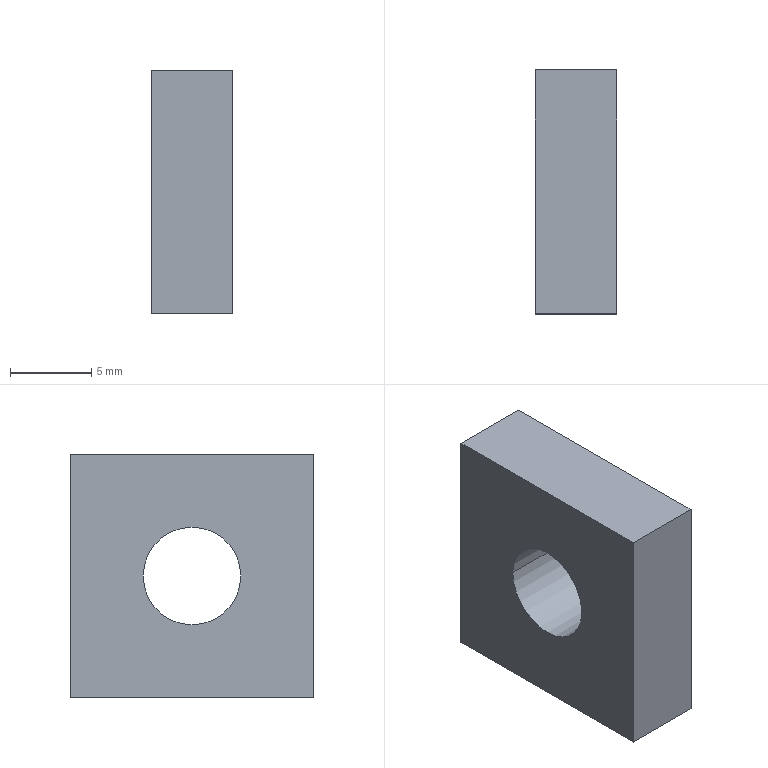Part | SolidWorks | features MBimport 1 | 1 solid | 8 faces | box 5 x 15 x 15 mm | volume 983.628 mm3 | plane 6 | cylinder 2 | commonest cylinder face diameters 6 x2
STEP:
#1=CARTESIAN_POINT('',(0.,3.,0.));
#2=VERTEX_POINT('',#1);
#3=CARTESIAN_POINT('',(0.,-3.,0.));
#4=VERTEX_POINT('',#3);
#5=CARTESIAN_POINT('',(0.,0.,0.));
#6=DIRECTION('',(-1.,0.,0.));
#7=DIRECTION('',(0.,1.,0.));
#8=AXIS2_PLACEMENT_3D('',#5,#6,#7);
#9=CIRCLE('',#8,3.);
#10=EDGE_CURVE('',#2,#4,#9,.T.);
#11=ORIENTED_EDGE('',*,*,#10,.F.);
#12=CARTESIAN_POINT('',(0.,0.,0.));
#13=DIRECTION('',(-1.,0.,0.));
#14=DIRECTION('',(0.,-1.,0.));
#15=AXIS2_PLACEMENT_3D('',#12,#13,#14);
#16=CIRCLE('',#15,3.);
#17=EDGE_CURVE('',#4,#2,#16,.T.);
#18=ORIENTED_EDGE('',*,*,#17,.F.);
#19=EDGE_LOOP('',(#11,#18));
#20=FACE_BOUND('',#19,.T.);
#21=CARTESIAN_POINT('',(0.,7.5,7.5));
#22=VERTEX_POINT('',#21);
#23=CARTESIAN_POINT('',(0.,-7.5,7.5));
#24=VERTEX_POINT('',#23);
#25=CARTESIAN_POINT('',(0.,7.5,7.5));
#26=DIRECTION('',(0.,-1.,0.));
#27=VECTOR('',#26,1000.);
#28=LINE('',#25,#27);
#29=EDGE_CURVE('',#22,#24,#28,.T.);
#30=ORIENTED_EDGE('',*,*,#29,.F.);
#31=CARTESIAN_POINT('',(0.,7.5,-7.5));
#32=VERTEX_POINT('',#31);
#33=CARTESIAN_POINT('',(0.,7.5,-7.5));
#34=DIRECTION('',(0.,0.,1.));
#35=VECTOR('',#34,1000.);
#36=LINE('',#33,#35);
#37=EDGE_CURVE('',#32,#22,#36,.T.);
#38=ORIENTED_EDGE('',*,*,#37,.F.);
#39=CARTESIAN_POINT('',(0.,-7.5,-7.5));
#40=VERTEX_POINT('',#39);
#41=CARTESIAN_POINT('',(0.,-7.5,-7.5));
#42=DIRECTION('',(0.,1.,0.));
#43=VECTOR('',#42,1000.);
#44=LINE('',#41,#43);
#45=EDGE_CURVE('',#40,#32,#44,.T.);
#46=ORIENTED_EDGE('',*,*,#45,.F.);
#47=CARTESIAN_POINT('',(0.,-7.5,7.5));
#48=DIRECTION('',(0.,0.,-1.));
#49=VECTOR('',#48,1000.);
#50=LINE('',#47,#49);
#51=EDGE_CURVE('',#24,#40,#50,.T.);
#52=ORIENTED_EDGE('',*,*,#51,.F.);
#53=EDGE_LOOP('',(#30,#38,#46,#52));
#54=FACE_OUTER_BOUND('',#53,.T.);
#55=CARTESIAN_POINT('',(0.,0.,0.));
#56=DIRECTION('',(1.,0.,0.));
#57=DIRECTION('',(0.,1.,0.));
#58=AXIS2_PLACEMENT_3D('',#55,#56,#57);
#59=PLANE('',#58);
#60=ADVANCED_FACE('',(#20,#54),#59,.F.);
#61=CARTESIAN_POINT('',(5.,-3.,0.));
#62=VERTEX_POINT('',#61);
#63=CARTESIAN_POINT('',(0.,-3.,0.));
#64=DIRECTION('',(1.,0.,0.));
#65=VECTOR('',#64,1000.);
#66=LINE('',#63,#65);
#67=EDGE_CURVE('',#4,#62,#66,.T.);
#68=ORIENTED_EDGE('',*,*,#67,.T.);
#69=CARTESIAN_POINT('',(5.,3.,0.));
#70=VERTEX_POINT('',#69);
#71=CARTESIAN_POINT('',(5.,0.,0.));
#72=DIRECTION('',(-1.,0.,0.));
#73=DIRECTION('',(0.,1.,0.));
#74=AXIS2_PLACEMENT_3D('',#71,#72,#73);
#75=CIRCLE('',#74,3.);
#76=EDGE_CURVE('',#70,#62,#75,.T.);
#77=ORIENTED_EDGE('',*,*,#76,.F.);
#78=CARTESIAN_POINT('',(0.,3.,0.));
#79=DIRECTION('',(1.,0.,0.));
#80=VECTOR('',#79,1000.);
#81=LINE('',#78,#80);
#82=EDGE_CURVE('',#2,#70,#81,.T.);
#83=ORIENTED_EDGE('',*,*,#82,.F.);
#84=ORIENTED_EDGE('',*,*,#10,.T.);
#85=EDGE_LOOP('',(#68,#77,#83,#84));
#86=FACE_OUTER_BOUND('',#85,.T.);
#87=CARTESIAN_POINT('',(0.,0.,0.));
#88=DIRECTION('',(1.,0.,0.));
#89=DIRECTION('',(0.,-1.,0.));
#90=AXIS2_PLACEMENT_3D('',#87,#88,#89);
#91=CYLINDRICAL_SURFACE('',#90,3.);
#92=ADVANCED_FACE('',(#86),#91,.F.);
#93=ORIENTED_EDGE('',*,*,#82,.T.);
#94=CARTESIAN_POINT('',(5.,0.,0.));
#95=DIRECTION('',(-1.,0.,0.));
#96=DIRECTION('',(0.,-1.,0.));
#97=AXIS2_PLACEMENT_3D('',#94,#95,#96);
#98=CIRCLE('',#97,3.);
#99=EDGE_CURVE('',#62,#70,#98,.T.);
#100=ORIENTED_EDGE('',*,*,#99,.F.);
#101=ORIENTED_EDGE('',*,*,#67,.F.);
#102=ORIENTED_EDGE('',*,*,#17,.T.);
#103=EDGE_LOOP('',(#93,#100,#101,#102));
#104=FACE_OUTER_BOUND('',#103,.T.);
#105=CARTESIAN_POINT('',(0.,0.,0.));
#106=DIRECTION('',(1.,0.,0.));
#107=DIRECTION('',(0.,-1.,0.));
#108=AXIS2_PLACEMENT_3D('',#105,#106,#107);
#109=CYLINDRICAL_SURFACE('',#108,3.);
#110=ADVANCED_FACE('',(#104),#109,.F.);
#111=CARTESIAN_POINT('',(5.,-7.5,7.5));
#112=VERTEX_POINT('',#111);
#113=CARTESIAN_POINT('',(0.,-7.5,7.5));
#114=DIRECTION('',(1.,0.,0.));
#115=VECTOR('',#114,1000.);
#116=LINE('',#113,#115);
#117=EDGE_CURVE('',#24,#112,#116,.T.);
#118=ORIENTED_EDGE('',*,*,#117,.T.);
#119=CARTESIAN_POINT('',(5.,7.5,7.5));
#120=VERTEX_POINT('',#119);
#121=CARTESIAN_POINT('',(5.,7.5,7.5));
#122=DIRECTION('',(0.,-1.,0.));
#123=VECTOR('',#122,1000.);
#124=LINE('',#121,#123);
#125=EDGE_CURVE('',#120,#112,#124,.T.);
#126=ORIENTED_EDGE('',*,*,#125,.F.);
#127=CARTESIAN_POINT('',(0.,7.5,7.5));
#128=DIRECTION('',(1.,0.,0.));
#129=VECTOR('',#128,1000.);
#130=LINE('',#127,#129);
#131=EDGE_CURVE('',#22,#120,#130,.T.);
#132=ORIENTED_EDGE('',*,*,#131,.F.);
#133=ORIENTED_EDGE('',*,*,#29,.T.);
#134=EDGE_LOOP('',(#118,#126,#132,#133));
#135=FACE_OUTER_BOUND('',#134,.T.);
#136=CARTESIAN_POINT('',(0.,7.5,7.5));
#137=DIRECTION('',(0.,0.,1.));
#138=DIRECTION('',(0.,-1.,0.));
#139=AXIS2_PLACEMENT_3D('',#136,#137,#138);
#140=PLANE('',#139);
#141=ADVANCED_FACE('',(#135),#140,.T.);
#142=ORIENTED_EDGE('',*,*,#131,.T.);
#143=CARTESIAN_POINT('',(5.,7.5,-7.5));
#144=VERTEX_POINT('',#143);
#145=CARTESIAN_POINT('',(5.,7.5,-7.5));
#146=DIRECTION('',(0.,0.,1.));
#147=VECTOR('',#146,1000.);
#148=LINE('',#145,#147);
#149=EDGE_CURVE('',#144,#120,#148,.T.);
#150=ORIENTED_EDGE('',*,*,#149,.F.);
#151=CARTESIAN_POINT('',(0.,7.5,-7.5));
#152=DIRECTION('',(1.,0.,0.));
#153=VECTOR('',#152,1000.);
#154=LINE('',#151,#153);
#155=EDGE_CURVE('',#32,#144,#154,.T.);
#156=ORIENTED_EDGE('',*,*,#155,.F.);
#157=ORIENTED_EDGE('',*,*,#37,.T.);
#158=EDGE_LOOP('',(#142,#150,#156,#157));
#159=FACE_OUTER_BOUND('',#158,.T.);
#160=CARTESIAN_POINT('',(0.,7.5,-7.5));
#161=DIRECTION('',(0.,1.,0.));
#162=DIRECTION('',(0.,0.,1.));
#163=AXIS2_PLACEMENT_3D('',#160,#161,#162);
#164=PLANE('',#163);
#165=ADVANCED_FACE('',(#159),#164,.T.);
#166=ORIENTED_EDGE('',*,*,#155,.T.);
#167=CARTESIAN_POINT('',(5.,-7.5,-7.5));
#168=VERTEX_POINT('',#167);
#169=CARTESIAN_POINT('',(5.,-7.5,-7.5));
#170=DIRECTION('',(0.,1.,0.));
#171=VECTOR('',#170,1000.);
#172=LINE('',#169,#171);
#173=EDGE_CURVE('',#168,#144,#172,.T.);
#174=ORIENTED_EDGE('',*,*,#173,.F.);
#175=CARTESIAN_POINT('',(0.,-7.5,-7.5));
#176=DIRECTION('',(1.,0.,0.));
#177=VECTOR('',#176,1000.);
#178=LINE('',#175,#177);
#179=EDGE_CURVE('',#40,#168,#178,.T.);
#180=ORIENTED_EDGE('',*,*,#179,.F.);
#181=ORIENTED_EDGE('',*,*,#45,.T.);
#182=EDGE_LOOP('',(#166,#174,#180,#181));
#183=FACE_OUTER_BOUND('',#182,.T.);
#184=CARTESIAN_POINT('',(0.,-7.5,-7.5));
#185=DIRECTION('',(0.,0.,-1.));
#186=DIRECTION('',(0.,1.,0.));
#187=AXIS2_PLACEMENT_3D('',#184,#185,#186);
#188=PLANE('',#187);
#189=ADVANCED_FACE('',(#183),#188,.T.);
#190=ORIENTED_EDGE('',*,*,#179,.T.);
#191=CARTESIAN_POINT('',(5.,-7.5,7.5));
#192=DIRECTION('',(0.,0.,-1.));
#193=VECTOR('',#192,1000.);
#194=LINE('',#191,#193);
#195=EDGE_CURVE('',#112,#168,#194,.T.);
#196=ORIENTED_EDGE('',*,*,#195,.F.);
#197=ORIENTED_EDGE('',*,*,#117,.F.);
#198=ORIENTED_EDGE('',*,*,#51,.T.);
#199=EDGE_LOOP('',(#190,#196,#197,#198));
#200=FACE_OUTER_BOUND('',#199,.T.);
#201=CARTESIAN_POINT('',(0.,-7.5,7.5));
#202=DIRECTION('',(0.,-1.,0.));
#203=DIRECTION('',(0.,0.,-1.));
#204=AXIS2_PLACEMENT_3D('',#201,#202,#203);
#205=PLANE('',#204);
#206=ADVANCED_FACE('',(#200),#205,.T.);
#207=ORIENTED_EDGE('',*,*,#76,.T.);
#208=ORIENTED_EDGE('',*,*,#99,.T.);
#209=EDGE_LOOP('',(#207,#208));
#210=FACE_BOUND('',#209,.T.);
#211=ORIENTED_EDGE('',*,*,#173,.T.);
#212=ORIENTED_EDGE('',*,*,#149,.T.);
#213=ORIENTED_EDGE('',*,*,#125,.T.);
#214=ORIENTED_EDGE('',*,*,#195,.T.);
#215=EDGE_LOOP('',(#211,#212,#213,#214));
#216=FACE_OUTER_BOUND('',#215,.T.);
#217=CARTESIAN_POINT('',(5.,0.,0.));
#218=DIRECTION('',(1.,0.,0.));
#219=DIRECTION('',(0.,1.,0.));
#220=AXIS2_PLACEMENT_3D('',#217,#218,#219);
#221=PLANE('',#220);
#222=ADVANCED_FACE('',(#210,#216),#221,.T.);
#223=CLOSED_SHELL('',(#60,#92,#110,#141,#165,#189,#206,#222));
#224=MANIFOLD_SOLID_BREP('',#223);
#225=CARTESIAN_POINT('',(0.,0.,0.));
#226=DIRECTION('',(0.,0.,1.));
#227=DIRECTION('',(1.,0.,0.));
#228=AXIS2_PLACEMENT_3D('',#225,#226,#227);
#229=(LENGTH_UNIT()NAMED_UNIT(*)SI_UNIT(.MILLI.,.METRE.));
#230=UNCERTAINTY_MEASURE_WITH_UNIT(LENGTH_MEASURE(0.00001),#229,'','');
#231=(NAMED_UNIT(*)PLANE_ANGLE_UNIT()SI_UNIT($,.RADIAN.));
#232=(NAMED_UNIT(*)SI_UNIT($,.STERADIAN.)SOLID_ANGLE_UNIT());
#233=(GEOMETRIC_REPRESENTATION_CONTEXT(3)GLOBAL_UNCERTAINTY_ASSIGNED_CONTEXT((#230))GLOBAL_UNIT_ASSIGNED_CONTEXT((#229,#231,#232))REPRESENTATION_CONTEXT('',''));
#234=ADVANCED_BREP_SHAPE_REPRESENTATION('',(#224,#228),#233);